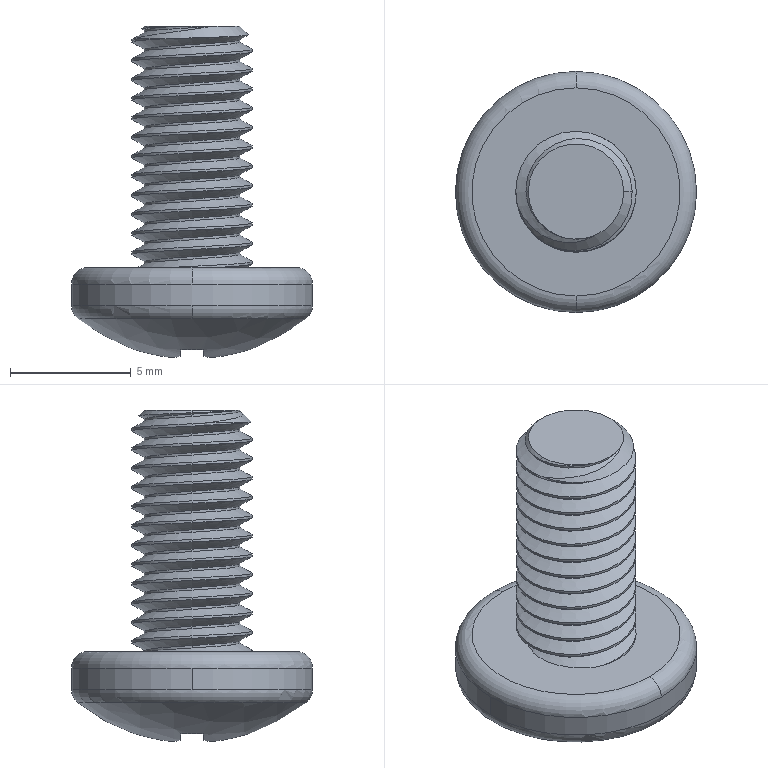Part | NX | features solid 2 | 1 solid | 89 faces | box 10 x 10 x 13.732 mm | volume 362.473 mm3 | cylinder 53 | plane 19 | cone 9 | torus 4 | spline 3 | sphere 1 | commonest cylinder face diameters 3.961 x26 5 x25 10 x2